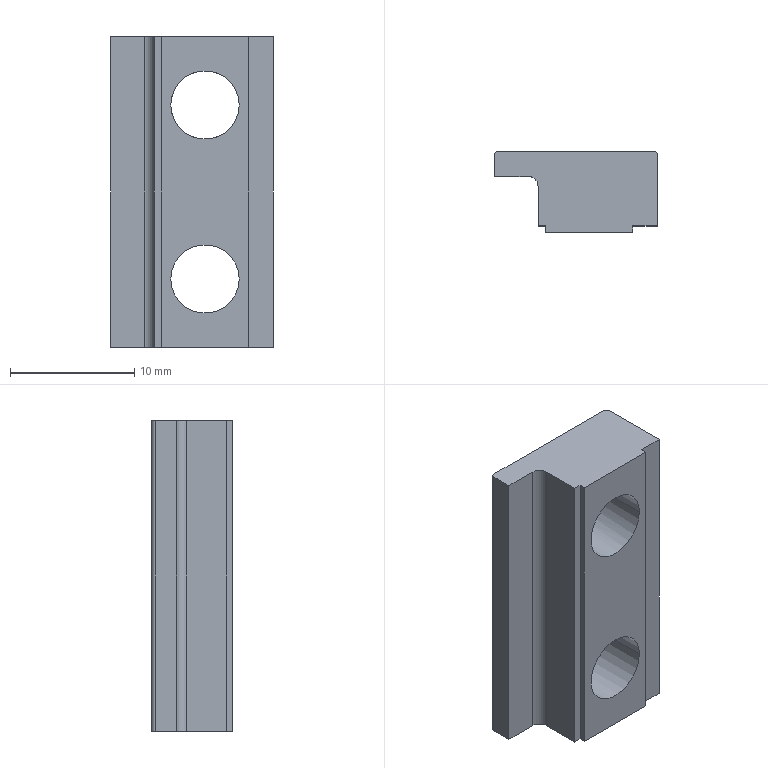Part | SolidWorks | features BaseBody 1 | 1 solid | 23 faces | box 13.1 x 6.5 x 25 mm | volume 1279 mm3 | plane 12 | cylinder 7 | cone 4 | commonest cylinder face diameters 5.5 x4 0.6 x2 1.6 x1
STEP:
#1=CARTESIAN_POINT('',(1.05,0.4528,4.25));
#2=VERTEX_POINT('',#1);
#3=CARTESIAN_POINT('',(-1.7,0.4528,7.));
#4=VERTEX_POINT('',#3);
#5=CARTESIAN_POINT('',(1.05,0.4528,7.));
#6=DIRECTION('',(0.,1.,0.));
#7=DIRECTION('',(0.,0.,1.));
#8=AXIS2_PLACEMENT_3D('',#5,#6,#7);
#9=CIRCLE('',#8,2.75);
#10=EDGE_CURVE('',#2,#4,#9,.T.);
#11=ORIENTED_EDGE('',*,*,#10,.F.);
#12=CARTESIAN_POINT('',(1.05,2.753,1.95));
#13=VERTEX_POINT('',#12);
#14=CARTESIAN_POINT('',(1.05,2.753,1.95));
#15=DIRECTION('',(0.,0.7071,-0.7071));
#16=VECTOR('',#15,1000.);
#17=LINE('',#14,#16);
#18=EDGE_CURVE('',#2,#13,#17,.T.);
#19=ORIENTED_EDGE('',*,*,#18,.T.);
#20=CARTESIAN_POINT('',(1.05,2.753,12.05));
#21=VERTEX_POINT('',#20);
#22=CARTESIAN_POINT('',(1.05,2.753,7.));
#23=DIRECTION('',(0.,-1.,0.));
#24=DIRECTION('',(0.,0.,1.));
#25=AXIS2_PLACEMENT_3D('',#22,#23,#24);
#26=CIRCLE('',#25,5.05);
#27=EDGE_CURVE('',#21,#13,#26,.T.);
#28=ORIENTED_EDGE('',*,*,#27,.F.);
#29=CARTESIAN_POINT('',(1.05,0.4528,9.75));
#30=VERTEX_POINT('',#29);
#31=CARTESIAN_POINT('',(1.05,2.753,12.05));
#32=DIRECTION('',(0.,0.7071,0.7071));
#33=VECTOR('',#32,1000.);
#34=LINE('',#31,#33);
#35=EDGE_CURVE('',#30,#21,#34,.T.);
#36=ORIENTED_EDGE('',*,*,#35,.F.);
#37=CARTESIAN_POINT('',(1.05,0.4528,7.));
#38=DIRECTION('',(0.,1.,0.));
#39=DIRECTION('',(0.,0.,1.));
#40=AXIS2_PLACEMENT_3D('',#37,#38,#39);
#41=CIRCLE('',#40,2.75);
#42=EDGE_CURVE('',#4,#30,#41,.T.);
#43=ORIENTED_EDGE('',*,*,#42,.F.);
#44=EDGE_LOOP('',(#11,#19,#28,#36,#43));
#45=FACE_OUTER_BOUND('',#44,.T.);
#46=CARTESIAN_POINT('',(1.05,2.753,7.));
#47=DIRECTION('',(0.,1.,0.));
#48=DIRECTION('',(0.,0.,1.));
#49=AXIS2_PLACEMENT_3D('',#46,#47,#48);
#50=CONICAL_SURFACE('',#49,5.05,0.7854);
#51=ADVANCED_FACE('',(#45),#50,.F.);
#52=CARTESIAN_POINT('',(3.8,0.4528,-7.));
#53=VERTEX_POINT('',#52);
#54=CARTESIAN_POINT('',(-1.7,0.4528,-7.));
#55=VERTEX_POINT('',#54);
#56=CARTESIAN_POINT('',(1.05,0.4528,-7.));
#57=DIRECTION('',(0.,1.,0.));
#58=DIRECTION('',(-1.,0.,0.));
#59=AXIS2_PLACEMENT_3D('',#56,#57,#58);
#60=CIRCLE('',#59,2.75);
#61=EDGE_CURVE('',#53,#55,#60,.T.);
#62=ORIENTED_EDGE('',*,*,#61,.F.);
#63=CARTESIAN_POINT('',(6.1,2.753,-7.));
#64=VERTEX_POINT('',#63);
#65=CARTESIAN_POINT('',(6.1,2.753,-7.));
#66=DIRECTION('',(0.7071,0.7071,0.));
#67=VECTOR('',#66,1000.);
#68=LINE('',#65,#67);
#69=EDGE_CURVE('',#53,#64,#68,.T.);
#70=ORIENTED_EDGE('',*,*,#69,.T.);
#71=CARTESIAN_POINT('',(-4.,2.753,-7.));
#72=VERTEX_POINT('',#71);
#73=CARTESIAN_POINT('',(1.05,2.753,-7.));
#74=DIRECTION('',(0.,-1.,0.));
#75=DIRECTION('',(-1.,0.,0.));
#76=AXIS2_PLACEMENT_3D('',#73,#74,#75);
#77=CIRCLE('',#76,5.05);
#78=EDGE_CURVE('',#72,#64,#77,.T.);
#79=ORIENTED_EDGE('',*,*,#78,.F.);
#80=CARTESIAN_POINT('',(-4.,2.753,-7.));
#81=DIRECTION('',(-0.7071,0.7071,0.));
#82=VECTOR('',#81,1000.);
#83=LINE('',#80,#82);
#84=EDGE_CURVE('',#55,#72,#83,.T.);
#85=ORIENTED_EDGE('',*,*,#84,.F.);
#86=EDGE_LOOP('',(#62,#70,#79,#85));
#87=FACE_OUTER_BOUND('',#86,.T.);
#88=CARTESIAN_POINT('',(1.05,2.753,-7.));
#89=DIRECTION('',(0.,1.,0.));
#90=DIRECTION('',(-1.,0.,0.));
#91=AXIS2_PLACEMENT_3D('',#88,#89,#90);
#92=CONICAL_SURFACE('',#91,5.05,0.7854);
#93=ADVANCED_FACE('',(#87),#92,.F.);
#94=CARTESIAN_POINT('',(3.8,0.4528,7.));
#95=VERTEX_POINT('',#94);
#96=CARTESIAN_POINT('',(1.05,0.4528,7.));
#97=DIRECTION('',(0.,1.,0.));
#98=DIRECTION('',(0.,0.,1.));
#99=AXIS2_PLACEMENT_3D('',#96,#97,#98);
#100=CIRCLE('',#99,2.75);
#101=EDGE_CURVE('',#95,#2,#100,.T.);
#102=ORIENTED_EDGE('',*,*,#101,.T.);
#103=ORIENTED_EDGE('',*,*,#10,.T.);
#104=CARTESIAN_POINT('',(-1.7,-3.747,7.));
#105=VERTEX_POINT('',#104);
#106=CARTESIAN_POINT('',(-1.7,-3.747,7.));
#107=DIRECTION('',(0.,-1.,0.));
#108=VECTOR('',#107,1000.);
#109=LINE('',#106,#108);
#110=EDGE_CURVE('',#4,#105,#109,.T.);
#111=ORIENTED_EDGE('',*,*,#110,.T.);
#112=CARTESIAN_POINT('',(3.8,-3.747,7.));
#113=VERTEX_POINT('',#112);
#114=CARTESIAN_POINT('',(1.05,-3.747,7.));
#115=DIRECTION('',(0.,1.,0.));
#116=DIRECTION('',(1.,0.,0.));
#117=AXIS2_PLACEMENT_3D('',#114,#115,#116);
#118=CIRCLE('',#117,2.75);
#119=EDGE_CURVE('',#113,#105,#118,.T.);
#120=ORIENTED_EDGE('',*,*,#119,.F.);
#121=CARTESIAN_POINT('',(3.8,-3.747,7.));
#122=DIRECTION('',(0.,-1.,0.));
#123=VECTOR('',#122,1000.);
#124=LINE('',#121,#123);
#125=EDGE_CURVE('',#95,#113,#124,.T.);
#126=ORIENTED_EDGE('',*,*,#125,.F.);
#127=EDGE_LOOP('',(#102,#103,#111,#120,#126));
#128=FACE_OUTER_BOUND('',#127,.T.);
#129=CARTESIAN_POINT('',(1.05,-3.747,7.));
#130=DIRECTION('',(0.,-1.,0.));
#131=DIRECTION('',(1.,0.,0.));
#132=AXIS2_PLACEMENT_3D('',#129,#130,#131);
#133=CYLINDRICAL_SURFACE('',#132,2.75);
#134=ADVANCED_FACE('',(#128),#133,.F.);
#135=ORIENTED_EDGE('',*,*,#61,.T.);
#136=CARTESIAN_POINT('',(-1.7,-3.747,-7.));
#137=VERTEX_POINT('',#136);
#138=CARTESIAN_POINT('',(-1.7,-3.747,-7.));
#139=DIRECTION('',(0.,-1.,0.));
#140=VECTOR('',#139,1000.);
#141=LINE('',#138,#140);
#142=EDGE_CURVE('',#55,#137,#141,.T.);
#143=ORIENTED_EDGE('',*,*,#142,.T.);
#144=CARTESIAN_POINT('',(3.8,-3.747,-7.));
#145=VERTEX_POINT('',#144);
#146=CARTESIAN_POINT('',(1.05,-3.747,-7.));
#147=DIRECTION('',(0.,1.,0.));
#148=DIRECTION('',(1.,0.,0.));
#149=AXIS2_PLACEMENT_3D('',#146,#147,#148);
#150=CIRCLE('',#149,2.75);
#151=EDGE_CURVE('',#145,#137,#150,.T.);
#152=ORIENTED_EDGE('',*,*,#151,.F.);
#153=CARTESIAN_POINT('',(3.8,-3.747,-7.));
#154=DIRECTION('',(0.,-1.,0.));
#155=VECTOR('',#154,1000.);
#156=LINE('',#153,#155);
#157=EDGE_CURVE('',#53,#145,#156,.T.);
#158=ORIENTED_EDGE('',*,*,#157,.F.);
#159=EDGE_LOOP('',(#135,#143,#152,#158));
#160=FACE_OUTER_BOUND('',#159,.T.);
#161=CARTESIAN_POINT('',(1.05,-3.747,-7.));
#162=DIRECTION('',(0.,-1.,0.));
#163=DIRECTION('',(1.,0.,0.));
#164=AXIS2_PLACEMENT_3D('',#161,#162,#163);
#165=CYLINDRICAL_SURFACE('',#164,2.75);
#166=ADVANCED_FACE('',(#160),#165,.F.);
#167=ORIENTED_EDGE('',*,*,#27,.T.);
#168=CARTESIAN_POINT('',(1.05,2.753,7.));
#169=DIRECTION('',(0.,-1.,0.));
#170=DIRECTION('',(0.,0.,1.));
#171=AXIS2_PLACEMENT_3D('',#168,#169,#170);
#172=CIRCLE('',#171,5.05);
#173=EDGE_CURVE('',#13,#21,#172,.T.);
#174=ORIENTED_EDGE('',*,*,#173,.T.);
#175=EDGE_LOOP('',(#167,#174));
#176=FACE_BOUND('',#175,.T.);
#177=ORIENTED_EDGE('',*,*,#78,.T.);
#178=CARTESIAN_POINT('',(1.05,2.753,-7.));
#179=DIRECTION('',(0.,-1.,0.));
#180=DIRECTION('',(-1.,0.,0.));
#181=AXIS2_PLACEMENT_3D('',#178,#179,#180);
#182=CIRCLE('',#181,5.05);
#183=EDGE_CURVE('',#64,#72,#182,.T.);
#184=ORIENTED_EDGE('',*,*,#183,.T.);
#185=EDGE_LOOP('',(#177,#184));
#186=FACE_BOUND('',#185,.T.);
#187=CARTESIAN_POINT('',(6.25,2.753,12.5));
#188=VERTEX_POINT('',#187);
#189=CARTESIAN_POINT('',(6.25,2.753,-12.5));
#190=VERTEX_POINT('',#189);
#191=CARTESIAN_POINT('',(6.25,2.753,-12.5));
#192=DIRECTION('',(0.,0.,-1.));
#193=VECTOR('',#192,1000.);
#194=LINE('',#191,#193);
#195=EDGE_CURVE('',#188,#190,#194,.T.);
#196=ORIENTED_EDGE('',*,*,#195,.T.);
#197=CARTESIAN_POINT('',(-6.25,2.753,-12.5));
#198=VERTEX_POINT('',#197);
#199=CARTESIAN_POINT('',(6.25,2.753,-12.5));
#200=DIRECTION('',(-1.,0.,0.));
#201=VECTOR('',#200,1000.);
#202=LINE('',#199,#201);
#203=EDGE_CURVE('',#190,#198,#202,.T.);
#204=ORIENTED_EDGE('',*,*,#203,.T.);
#205=CARTESIAN_POINT('',(-6.25,2.753,12.5));
#206=VERTEX_POINT('',#205);
#207=CARTESIAN_POINT('',(-6.25,2.753,-12.5));
#208=DIRECTION('',(0.,0.,1.));
#209=VECTOR('',#208,1000.);
#210=LINE('',#207,#209);
#211=EDGE_CURVE('',#198,#206,#210,.T.);
#212=ORIENTED_EDGE('',*,*,#211,.T.);
#213=CARTESIAN_POINT('',(6.25,2.753,12.5));
#214=DIRECTION('',(1.,0.,0.));
#215=VECTOR('',#214,1000.);
#216=LINE('',#213,#215);
#217=EDGE_CURVE('',#206,#188,#216,.T.);
#218=ORIENTED_EDGE('',*,*,#217,.T.);
#219=EDGE_LOOP('',(#196,#204,#212,#218));
#220=FACE_OUTER_BOUND('',#219,.T.);
#221=CARTESIAN_POINT('',(6.25,2.753,-12.5));
#222=DIRECTION('',(0.,1.,0.));
#223=DIRECTION('',(-1.,0.,0.));
#224=AXIS2_PLACEMENT_3D('',#221,#222,#223);
#225=PLANE('',#224);
#226=ADVANCED_FACE('',(#176,#186,#220),#225,.T.);
#227=ORIENTED_EDGE('',*,*,#18,.F.);
#228=ORIENTED_EDGE('',*,*,#101,.F.);
#229=CARTESIAN_POINT('',(1.05,0.4528,7.));
#230=DIRECTION('',(0.,1.,0.));
#231=DIRECTION('',(0.,0.,1.));
#232=AXIS2_PLACEMENT_3D('',#229,#230,#231);
#233=CIRCLE('',#232,2.75);
#234=EDGE_CURVE('',#30,#95,#233,.T.);
#235=ORIENTED_EDGE('',*,*,#234,.F.);
#236=ORIENTED_EDGE('',*,*,#35,.T.);
#237=ORIENTED_EDGE('',*,*,#173,.F.);
#238=EDGE_LOOP('',(#227,#228,#235,#236,#237));
#239=FACE_OUTER_BOUND('',#238,.T.);
#240=CARTESIAN_POINT('',(1.05,2.753,7.));
#241=DIRECTION('',(0.,1.,0.));
#242=DIRECTION('',(0.,0.,1.));
#243=AXIS2_PLACEMENT_3D('',#240,#241,#242);
#244=CONICAL_SURFACE('',#243,5.05,0.7854);
#245=ADVANCED_FACE('',(#239),#244,.F.);
#246=ORIENTED_EDGE('',*,*,#69,.F.);
#247=CARTESIAN_POINT('',(1.05,0.4528,-7.));
#248=DIRECTION('',(0.,1.,0.));
#249=DIRECTION('',(-1.,0.,0.));
#250=AXIS2_PLACEMENT_3D('',#247,#248,#249);
#251=CIRCLE('',#250,2.75);
#252=EDGE_CURVE('',#55,#53,#251,.T.);
#253=ORIENTED_EDGE('',*,*,#252,.F.);
#254=ORIENTED_EDGE('',*,*,#84,.T.);
#255=ORIENTED_EDGE('',*,*,#183,.F.);
#256=EDGE_LOOP('',(#246,#253,#254,#255));
#257=FACE_OUTER_BOUND('',#256,.T.);
#258=CARTESIAN_POINT('',(1.05,2.753,-7.));
#259=DIRECTION('',(0.,1.,0.));
#260=DIRECTION('',(-1.,0.,0.));
#261=AXIS2_PLACEMENT_3D('',#258,#259,#260);
#262=CONICAL_SURFACE('',#261,5.05,0.7854);
#263=ADVANCED_FACE('',(#257),#262,.F.);
#264=CARTESIAN_POINT('',(-3.05,-3.247,-12.5));
#265=VERTEX_POINT('',#264);
#266=CARTESIAN_POINT('',(-2.45,-3.247,-12.5));
#267=VERTEX_POINT('',#266);
#268=CARTESIAN_POINT('',(-3.05,-3.247,-12.5));
#269=DIRECTION('',(1.,0.,0.));
#270=VECTOR('',#269,1000.);
#271=LINE('',#268,#270);
#272=EDGE_CURVE('',#265,#267,#271,.T.);
#273=ORIENTED_EDGE('',*,*,#272,.F.);
#274=CARTESIAN_POINT('',(-3.05,-0.04716,-12.5));
#275=VERTEX_POINT('',#274);
#276=CARTESIAN_POINT('',(-3.05,0.,-12.5));
#277=DIRECTION('',(0.,-1.,0.));
#278=VECTOR('',#277,1000.);
#279=LINE('',#276,#278);
#280=EDGE_CURVE('',#275,#265,#279,.T.);
#281=ORIENTED_EDGE('',*,*,#280,.F.);
#282=CARTESIAN_POINT('',(-3.85,0.7528,-12.5));
#283=VERTEX_POINT('',#282);
#284=CARTESIAN_POINT('',(-3.85,-0.04716,-12.5));
#285=DIRECTION('',(0.,0.,1.));
#286=DIRECTION('',(0.,-1.,0.));
#287=AXIS2_PLACEMENT_3D('',#284,#285,#286);
#288=CIRCLE('',#287,0.8);
#289=EDGE_CURVE('',#275,#283,#288,.T.);
#290=ORIENTED_EDGE('',*,*,#289,.T.);
#291=CARTESIAN_POINT('',(-6.55,0.7528,-12.5));
#292=VERTEX_POINT('',#291);
#293=CARTESIAN_POINT('',(0.,0.7528,-12.5));
#294=DIRECTION('',(1.,0.,0.));
#295=VECTOR('',#294,1000.);
#296=LINE('',#293,#295);
#297=EDGE_CURVE('',#292,#283,#296,.T.);
#298=ORIENTED_EDGE('',*,*,#297,.F.);
#299=CARTESIAN_POINT('',(-6.55,2.453,-12.5));
#300=VERTEX_POINT('',#299);
#301=CARTESIAN_POINT('',(-6.55,2.453,-12.5));
#302=DIRECTION('',(0.,-1.,0.));
#303=VECTOR('',#302,1000.);
#304=LINE('',#301,#303);
#305=EDGE_CURVE('',#300,#292,#304,.T.);
#306=ORIENTED_EDGE('',*,*,#305,.F.);
#307=CARTESIAN_POINT('',(-6.25,2.453,-12.5));
#308=DIRECTION('',(0.,0.,1.));
#309=DIRECTION('',(0.,-1.,0.));
#310=AXIS2_PLACEMENT_3D('',#307,#308,#309);
#311=CIRCLE('',#310,0.3);
#312=EDGE_CURVE('',#198,#300,#311,.T.);
#313=ORIENTED_EDGE('',*,*,#312,.F.);
#314=ORIENTED_EDGE('',*,*,#203,.F.);
#315=CARTESIAN_POINT('',(6.55,2.453,-12.5));
#316=VERTEX_POINT('',#315);
#317=CARTESIAN_POINT('',(6.25,2.453,-12.5));
#318=DIRECTION('',(0.,0.,1.));
#319=DIRECTION('',(0.,-1.,0.));
#320=AXIS2_PLACEMENT_3D('',#317,#318,#319);
#321=CIRCLE('',#320,0.3);
#322=EDGE_CURVE('',#316,#190,#321,.T.);
#323=ORIENTED_EDGE('',*,*,#322,.F.);
#324=CARTESIAN_POINT('',(6.55,-3.247,-12.5));
#325=VERTEX_POINT('',#324);
#326=CARTESIAN_POINT('',(6.55,0.,-12.5));
#327=DIRECTION('',(0.,1.,0.));
#328=VECTOR('',#327,1000.);
#329=LINE('',#326,#328);
#330=EDGE_CURVE('',#325,#316,#329,.T.);
#331=ORIENTED_EDGE('',*,*,#330,.F.);
#332=CARTESIAN_POINT('',(4.55,-3.247,-12.5));
#333=VERTEX_POINT('',#332);
#334=CARTESIAN_POINT('',(0.,-3.247,-12.5));
#335=DIRECTION('',(1.,0.,0.));
#336=VECTOR('',#335,1000.);
#337=LINE('',#334,#336);
#338=EDGE_CURVE('',#333,#325,#337,.T.);
#339=ORIENTED_EDGE('',*,*,#338,.F.);
#340=CARTESIAN_POINT('',(4.55,-3.747,-12.5));
#341=VERTEX_POINT('',#340);
#342=CARTESIAN_POINT('',(4.55,-3.747,-12.5));
#343=DIRECTION('',(0.,1.,0.));
#344=VECTOR('',#343,1000.);
#345=LINE('',#342,#344);
#346=EDGE_CURVE('',#341,#333,#345,.T.);
#347=ORIENTED_EDGE('',*,*,#346,.F.);
#348=CARTESIAN_POINT('',(-2.45,-3.747,-12.5));
#349=VERTEX_POINT('',#348);
#350=CARTESIAN_POINT('',(0.,-3.747,-12.5));
#351=DIRECTION('',(1.,0.,0.));
#352=VECTOR('',#351,1000.);
#353=LINE('',#350,#352);
#354=EDGE_CURVE('',#349,#341,#353,.T.);
#355=ORIENTED_EDGE('',*,*,#354,.F.);
#356=CARTESIAN_POINT('',(-2.45,-3.247,-12.5));
#357=DIRECTION('',(0.,-1.,0.));
#358=VECTOR('',#357,1000.);
#359=LINE('',#356,#358);
#360=EDGE_CURVE('',#267,#349,#359,.T.);
#361=ORIENTED_EDGE('',*,*,#360,.F.);
#362=EDGE_LOOP('',(#273,#281,#290,#298,#306,#313,#314,#323,#331,#339,#347,#355,#361));
#363=FACE_OUTER_BOUND('',#362,.T.);
#364=CARTESIAN_POINT('',(0.,0.,-12.5));
#365=DIRECTION('',(0.,0.,1.));
#366=DIRECTION('',(0.,-1.,0.));
#367=AXIS2_PLACEMENT_3D('',#364,#365,#366);
#368=PLANE('',#367);
#369=ADVANCED_FACE('',(#363),#368,.F.);
#370=CARTESIAN_POINT('',(6.55,2.453,12.5));
#371=VERTEX_POINT('',#370);
#372=CARTESIAN_POINT('',(6.55,2.453,-12.5));
#373=DIRECTION('',(0.,0.,-1.));
#374=VECTOR('',#373,1000.);
#375=LINE('',#372,#374);
#376=EDGE_CURVE('',#371,#316,#375,.T.);
#377=ORIENTED_EDGE('',*,*,#376,.T.);
#378=ORIENTED_EDGE('',*,*,#322,.T.);
#379=ORIENTED_EDGE('',*,*,#195,.F.);
#380=CARTESIAN_POINT('',(6.25,2.453,12.5));
#381=DIRECTION('',(0.,0.,-1.));
#382=DIRECTION('',(0.,-1.,0.));
#383=AXIS2_PLACEMENT_3D('',#380,#381,#382);
#384=CIRCLE('',#383,0.3);
#385=EDGE_CURVE('',#188,#371,#384,.T.);
#386=ORIENTED_EDGE('',*,*,#385,.T.);
#387=EDGE_LOOP('',(#377,#378,#379,#386));
#388=FACE_OUTER_BOUND('',#387,.T.);
#389=CARTESIAN_POINT('',(6.25,2.453,-12.5));
#390=DIRECTION('',(0.,0.,1.));
#391=DIRECTION('',(0.,-1.,0.));
#392=AXIS2_PLACEMENT_3D('',#389,#390,#391);
#393=CYLINDRICAL_SURFACE('',#392,0.3);
#394=ADVANCED_FACE('',(#388),#393,.T.);
#395=CARTESIAN_POINT('',(-3.05,-0.04716,12.5));
#396=VERTEX_POINT('',#395);
#397=CARTESIAN_POINT('',(-3.05,-3.247,12.5));
#398=VERTEX_POINT('',#397);
#399=CARTESIAN_POINT('',(-3.05,0.,12.5));
#400=DIRECTION('',(0.,-1.,0.));
#401=VECTOR('',#400,1000.);
#402=LINE('',#399,#401);
#403=EDGE_CURVE('',#396,#398,#402,.T.);
#404=ORIENTED_EDGE('',*,*,#403,.T.);
#405=CARTESIAN_POINT('',(-2.45,-3.247,12.5));
#406=VERTEX_POINT('',#405);
#407=CARTESIAN_POINT('',(-3.05,-3.247,12.5));
#408=DIRECTION('',(-1.,0.,0.));
#409=VECTOR('',#408,1000.);
#410=LINE('',#407,#409);
#411=EDGE_CURVE('',#406,#398,#410,.T.);
#412=ORIENTED_EDGE('',*,*,#411,.F.);
#413=CARTESIAN_POINT('',(-2.45,-3.747,12.5));
#414=VERTEX_POINT('',#413);
#415=CARTESIAN_POINT('',(-2.45,-3.247,12.5));
#416=DIRECTION('',(0.,1.,0.));
#417=VECTOR('',#416,1000.);
#418=LINE('',#415,#417);
#419=EDGE_CURVE('',#414,#406,#418,.T.);
#420=ORIENTED_EDGE('',*,*,#419,.F.);
#421=CARTESIAN_POINT('',(4.55,-3.747,12.5));
#422=VERTEX_POINT('',#421);
#423=CARTESIAN_POINT('',(0.,-3.747,12.5));
#424=DIRECTION('',(1.,0.,0.));
#425=VECTOR('',#424,1000.);
#426=LINE('',#423,#425);
#427=EDGE_CURVE('',#414,#422,#426,.T.);
#428=ORIENTED_EDGE('',*,*,#427,.T.);
#429=CARTESIAN_POINT('',(4.55,-3.247,12.5));
#430=VERTEX_POINT('',#429);
#431=CARTESIAN_POINT('',(4.55,-3.747,12.5));
#432=DIRECTION('',(0.,-1.,0.));
#433=VECTOR('',#432,1000.);
#434=LINE('',#431,#433);
#435=EDGE_CURVE('',#430,#422,#434,.T.);
#436=ORIENTED_EDGE('',*,*,#435,.F.);
#437=CARTESIAN_POINT('',(6.55,-3.247,12.5));
#438=VERTEX_POINT('',#437);
#439=CARTESIAN_POINT('',(0.,-3.247,12.5));
#440=DIRECTION('',(1.,0.,0.));
#441=VECTOR('',#440,1000.);
#442=LINE('',#439,#441);
#443=EDGE_CURVE('',#430,#438,#442,.T.);
#444=ORIENTED_EDGE('',*,*,#443,.T.);
#445=CARTESIAN_POINT('',(6.55,0.,12.5));
#446=DIRECTION('',(0.,1.,0.));
#447=VECTOR('',#446,1000.);
#448=LINE('',#445,#447);
#449=EDGE_CURVE('',#438,#371,#448,.T.);
#450=ORIENTED_EDGE('',*,*,#449,.T.);
#451=ORIENTED_EDGE('',*,*,#385,.F.);
#452=ORIENTED_EDGE('',*,*,#217,.F.);
#453=CARTESIAN_POINT('',(-6.55,2.453,12.5));
#454=VERTEX_POINT('',#453);
#455=CARTESIAN_POINT('',(-6.25,2.453,12.5));
#456=DIRECTION('',(0.,0.,1.));
#457=DIRECTION('',(0.,-1.,0.));
#458=AXIS2_PLACEMENT_3D('',#455,#456,#457);
#459=CIRCLE('',#458,0.3);
#460=EDGE_CURVE('',#206,#454,#459,.T.);
#461=ORIENTED_EDGE('',*,*,#460,.T.);
#462=CARTESIAN_POINT('',(-6.55,0.7528,12.5));
#463=VERTEX_POINT('',#462);
#464=CARTESIAN_POINT('',(-6.55,2.453,12.5));
#465=DIRECTION('',(0.,1.,0.));
#466=VECTOR('',#465,1000.);
#467=LINE('',#464,#466);
#468=EDGE_CURVE('',#463,#454,#467,.T.);
#469=ORIENTED_EDGE('',*,*,#468,.F.);
#470=CARTESIAN_POINT('',(-3.85,0.7528,12.5));
#471=VERTEX_POINT('',#470);
#472=CARTESIAN_POINT('',(0.,0.7528,12.5));
#473=DIRECTION('',(1.,0.,0.));
#474=VECTOR('',#473,1000.);
#475=LINE('',#472,#474);
#476=EDGE_CURVE('',#463,#471,#475,.T.);
#477=ORIENTED_EDGE('',*,*,#476,.T.);
#478=CARTESIAN_POINT('',(-3.85,-0.04716,12.5));
#479=DIRECTION('',(0.,0.,-1.));
#480=DIRECTION('',(0.,-1.,0.));
#481=AXIS2_PLACEMENT_3D('',#478,#479,#480);
#482=CIRCLE('',#481,0.8);
#483=EDGE_CURVE('',#471,#396,#482,.T.);
#484=ORIENTED_EDGE('',*,*,#483,.T.);
#485=EDGE_LOOP('',(#404,#412,#420,#428,#436,#444,#450,#451,#452,#461,#469,#477,#484));
#486=FACE_OUTER_BOUND('',#485,.T.);
#487=CARTESIAN_POINT('',(0.,0.,12.5));
#488=DIRECTION('',(0.,0.,1.));
#489=DIRECTION('',(0.,-1.,0.));
#490=AXIS2_PLACEMENT_3D('',#487,#488,#489);
#491=PLANE('',#490);
#492=ADVANCED_FACE('',(#486),#491,.T.);
#493=ORIENTED_EDGE('',*,*,#211,.F.);
#494=ORIENTED_EDGE('',*,*,#312,.T.);
#495=CARTESIAN_POINT('',(-6.55,2.453,-12.5));
#496=DIRECTION('',(0.,0.,1.));
#497=VECTOR('',#496,1000.);
#498=LINE('',#495,#497);
#499=EDGE_CURVE('',#300,#454,#498,.T.);
#500=ORIENTED_EDGE('',*,*,#499,.T.);
#501=ORIENTED_EDGE('',*,*,#460,.F.);
#502=EDGE_LOOP('',(#493,#494,#500,#501));
#503=FACE_OUTER_BOUND('',#502,.T.);
#504=CARTESIAN_POINT('',(-6.25,2.453,-12.5));
#505=DIRECTION('',(0.,0.,1.));
#506=DIRECTION('',(0.,-1.,0.));
#507=AXIS2_PLACEMENT_3D('',#504,#505,#506);
#508=CYLINDRICAL_SURFACE('',#507,0.3);
#509=ADVANCED_FACE('',(#503),#508,.T.);
#510=ORIENTED_EDGE('',*,*,#110,.F.);
#511=ORIENTED_EDGE('',*,*,#42,.T.);
#512=ORIENTED_EDGE('',*,*,#234,.T.);
#513=ORIENTED_EDGE('',*,*,#125,.T.);
#514=CARTESIAN_POINT('',(1.05,-3.747,7.));
#515=DIRECTION('',(0.,1.,0.));
#516=DIRECTION('',(1.,0.,0.));
#517=AXIS2_PLACEMENT_3D('',#514,#515,#516);
#518=CIRCLE('',#517,2.75);
#519=EDGE_CURVE('',#105,#113,#518,.T.);
#520=ORIENTED_EDGE('',*,*,#519,.F.);
#521=EDGE_LOOP('',(#510,#511,#512,#513,#520));
#522=FACE_OUTER_BOUND('',#521,.T.);
#523=CARTESIAN_POINT('',(1.05,-3.747,7.));
#524=DIRECTION('',(0.,-1.,0.));
#525=DIRECTION('',(1.,0.,0.));
#526=AXIS2_PLACEMENT_3D('',#523,#524,#525);
#527=CYLINDRICAL_SURFACE('',#526,2.75);
#528=ADVANCED_FACE('',(#522),#527,.F.);
#529=ORIENTED_EDGE('',*,*,#142,.F.);
#530=ORIENTED_EDGE('',*,*,#252,.T.);
#531=ORIENTED_EDGE('',*,*,#157,.T.);
#532=CARTESIAN_POINT('',(1.05,-3.747,-7.));
#533=DIRECTION('',(0.,1.,0.));
#534=DIRECTION('',(1.,0.,0.));
#535=AXIS2_PLACEMENT_3D('',#532,#533,#534);
#536=CIRCLE('',#535,2.75);
#537=EDGE_CURVE('',#137,#145,#536,.T.);
#538=ORIENTED_EDGE('',*,*,#537,.F.);
#539=EDGE_LOOP('',(#529,#530,#531,#538));
#540=FACE_OUTER_BOUND('',#539,.T.);
#541=CARTESIAN_POINT('',(1.05,-3.747,-7.));
#542=DIRECTION('',(0.,-1.,0.));
#543=DIRECTION('',(1.,0.,0.));
#544=AXIS2_PLACEMENT_3D('',#541,#542,#543);
#545=CYLINDRICAL_SURFACE('',#544,2.75);
#546=ADVANCED_FACE('',(#540),#545,.F.);
#547=CARTESIAN_POINT('',(-3.05,-0.04716,-12.5));
#548=DIRECTION('',(0.,0.,-1.));
#549=VECTOR('',#548,1000.);
#550=LINE('',#547,#549);
#551=EDGE_CURVE('',#396,#275,#550,.T.);
#552=ORIENTED_EDGE('',*,*,#551,.T.);
#553=ORIENTED_EDGE('',*,*,#280,.T.);
#554=CARTESIAN_POINT('',(-3.05,-3.247,-12.5));
#555=DIRECTION('',(0.,0.,1.));
#556=VECTOR('',#555,1000.);
#557=LINE('',#554,#556);
#558=EDGE_CURVE('',#265,#398,#557,.T.);
#559=ORIENTED_EDGE('',*,*,#558,.T.);
#560=ORIENTED_EDGE('',*,*,#403,.F.);
#561=EDGE_LOOP('',(#552,#553,#559,#560));
#562=FACE_OUTER_BOUND('',#561,.T.);
#563=CARTESIAN_POINT('',(-3.05,-0.04716,-12.5));
#564=DIRECTION('',(-1.,0.,0.));
#565=DIRECTION('',(0.,-1.,0.));
#566=AXIS2_PLACEMENT_3D('',#563,#564,#565);
#567=PLANE('',#566);
#568=ADVANCED_FACE('',(#562),#567,.T.);
#569=CARTESIAN_POINT('',(-6.55,0.7528,-12.5));
#570=DIRECTION('',(0.,0.,-1.));
#571=VECTOR('',#570,1000.);
#572=LINE('',#569,#571);
#573=EDGE_CURVE('',#463,#292,#572,.T.);
#574=ORIENTED_EDGE('',*,*,#573,.T.);
#575=ORIENTED_EDGE('',*,*,#297,.T.);
#576=CARTESIAN_POINT('',(-3.85,0.7528,-12.5));
#577=DIRECTION('',(0.,0.,1.));
#578=VECTOR('',#577,1000.);
#579=LINE('',#576,#578);
#580=EDGE_CURVE('',#283,#471,#579,.T.);
#581=ORIENTED_EDGE('',*,*,#580,.T.);
#582=ORIENTED_EDGE('',*,*,#476,.F.);
#583=EDGE_LOOP('',(#574,#575,#581,#582));
#584=FACE_OUTER_BOUND('',#583,.T.);
#585=CARTESIAN_POINT('',(-6.55,0.7528,-12.5));
#586=DIRECTION('',(0.,-1.,0.));
#587=DIRECTION('',(1.,0.,0.));
#588=AXIS2_PLACEMENT_3D('',#585,#586,#587);
#589=PLANE('',#588);
#590=ADVANCED_FACE('',(#584),#589,.T.);
#591=CARTESIAN_POINT('',(6.55,-3.247,-12.5));
#592=DIRECTION('',(0.,0.,-1.));
#593=VECTOR('',#592,1000.);
#594=LINE('',#591,#593);
#595=EDGE_CURVE('',#438,#325,#594,.T.);
#596=ORIENTED_EDGE('',*,*,#595,.T.);
#597=ORIENTED_EDGE('',*,*,#330,.T.);
#598=ORIENTED_EDGE('',*,*,#376,.F.);
#599=ORIENTED_EDGE('',*,*,#449,.F.);
#600=EDGE_LOOP('',(#596,#597,#598,#599));
#601=FACE_OUTER_BOUND('',#600,.T.);
#602=CARTESIAN_POINT('',(6.55,-3.247,-12.5));
#603=DIRECTION('',(1.,0.,0.));
#604=DIRECTION('',(0.,1.,0.));
#605=AXIS2_PLACEMENT_3D('',#602,#603,#604);
#606=PLANE('',#605);
#607=ADVANCED_FACE('',(#601),#606,.T.);
#608=CARTESIAN_POINT('',(4.55,-3.247,-12.5));
#609=DIRECTION('',(0.,0.,-1.));
#610=VECTOR('',#609,1000.);
#611=LINE('',#608,#610);
#612=EDGE_CURVE('',#430,#333,#611,.T.);
#613=ORIENTED_EDGE('',*,*,#612,.T.);
#614=ORIENTED_EDGE('',*,*,#338,.T.);
#615=ORIENTED_EDGE('',*,*,#595,.F.);
#616=ORIENTED_EDGE('',*,*,#443,.F.);
#617=EDGE_LOOP('',(#613,#614,#615,#616));
#618=FACE_OUTER_BOUND('',#617,.T.);
#619=CARTESIAN_POINT('',(4.55,-3.247,-12.5));
#620=DIRECTION('',(0.,-1.,0.));
#621=DIRECTION('',(1.,0.,0.));
#622=AXIS2_PLACEMENT_3D('',#619,#620,#621);
#623=PLANE('',#622);
#624=ADVANCED_FACE('',(#618),#623,.T.);
#625=ORIENTED_EDGE('',*,*,#151,.T.);
#626=ORIENTED_EDGE('',*,*,#537,.T.);
#627=EDGE_LOOP('',(#625,#626));
#628=FACE_BOUND('',#627,.T.);
#629=ORIENTED_EDGE('',*,*,#119,.T.);
#630=ORIENTED_EDGE('',*,*,#519,.T.);
#631=EDGE_LOOP('',(#629,#630));
#632=FACE_BOUND('',#631,.T.);
#633=CARTESIAN_POINT('',(-2.45,-3.747,-12.5));
#634=DIRECTION('',(0.,0.,-1.));
#635=VECTOR('',#634,1000.);
#636=LINE('',#633,#635);
#637=EDGE_CURVE('',#414,#349,#636,.T.);
#638=ORIENTED_EDGE('',*,*,#637,.T.);
#639=ORIENTED_EDGE('',*,*,#354,.T.);
#640=CARTESIAN_POINT('',(4.55,-3.747,-12.5));
#641=DIRECTION('',(0.,0.,1.));
#642=VECTOR('',#641,1000.);
#643=LINE('',#640,#642);
#644=EDGE_CURVE('',#341,#422,#643,.T.);
#645=ORIENTED_EDGE('',*,*,#644,.T.);
#646=ORIENTED_EDGE('',*,*,#427,.F.);
#647=EDGE_LOOP('',(#638,#639,#645,#646));
#648=FACE_OUTER_BOUND('',#647,.T.);
#649=CARTESIAN_POINT('',(-2.45,-3.747,-12.5));
#650=DIRECTION('',(0.,-1.,0.));
#651=DIRECTION('',(1.,0.,0.));
#652=AXIS2_PLACEMENT_3D('',#649,#650,#651);
#653=PLANE('',#652);
#654=ADVANCED_FACE('',(#628,#632,#648),#653,.T.);
#655=ORIENTED_EDGE('',*,*,#499,.F.);
#656=ORIENTED_EDGE('',*,*,#305,.T.);
#657=ORIENTED_EDGE('',*,*,#573,.F.);
#658=ORIENTED_EDGE('',*,*,#468,.T.);
#659=EDGE_LOOP('',(#655,#656,#657,#658));
#660=FACE_OUTER_BOUND('',#659,.T.);
#661=CARTESIAN_POINT('',(-6.55,2.453,-12.5));
#662=DIRECTION('',(-1.,0.,0.));
#663=DIRECTION('',(0.,-1.,0.));
#664=AXIS2_PLACEMENT_3D('',#661,#662,#663);
#665=PLANE('',#664);
#666=ADVANCED_FACE('',(#660),#665,.T.);
#667=ORIENTED_EDGE('',*,*,#289,.F.);
#668=ORIENTED_EDGE('',*,*,#551,.F.);
#669=ORIENTED_EDGE('',*,*,#483,.F.);
#670=ORIENTED_EDGE('',*,*,#580,.F.);
#671=EDGE_LOOP('',(#667,#668,#669,#670));
#672=FACE_OUTER_BOUND('',#671,.T.);
#673=CARTESIAN_POINT('',(-3.85,-0.04716,-12.5));
#674=DIRECTION('',(0.,0.,1.));
#675=DIRECTION('',(0.,-1.,0.));
#676=AXIS2_PLACEMENT_3D('',#673,#674,#675);
#677=CYLINDRICAL_SURFACE('',#676,0.8);
#678=ADVANCED_FACE('',(#672),#677,.F.);
#679=ORIENTED_EDGE('',*,*,#558,.F.);
#680=ORIENTED_EDGE('',*,*,#272,.T.);
#681=CARTESIAN_POINT('',(-2.45,-3.247,-12.5));
#682=DIRECTION('',(0.,0.,1.));
#683=VECTOR('',#682,1000.);
#684=LINE('',#681,#683);
#685=EDGE_CURVE('',#267,#406,#684,.T.);
#686=ORIENTED_EDGE('',*,*,#685,.T.);
#687=ORIENTED_EDGE('',*,*,#411,.T.);
#688=EDGE_LOOP('',(#679,#680,#686,#687));
#689=FACE_OUTER_BOUND('',#688,.T.);
#690=CARTESIAN_POINT('',(-3.05,-3.247,-12.5));
#691=DIRECTION('',(0.,-1.,0.));
#692=DIRECTION('',(1.,0.,0.));
#693=AXIS2_PLACEMENT_3D('',#690,#691,#692);
#694=PLANE('',#693);
#695=ADVANCED_FACE('',(#689),#694,.T.);
#696=ORIENTED_EDGE('',*,*,#644,.F.);
#697=ORIENTED_EDGE('',*,*,#346,.T.);
#698=ORIENTED_EDGE('',*,*,#612,.F.);
#699=ORIENTED_EDGE('',*,*,#435,.T.);
#700=EDGE_LOOP('',(#696,#697,#698,#699));
#701=FACE_OUTER_BOUND('',#700,.T.);
#702=CARTESIAN_POINT('',(4.55,-3.747,-12.5));
#703=DIRECTION('',(1.,0.,0.));
#704=DIRECTION('',(0.,1.,0.));
#705=AXIS2_PLACEMENT_3D('',#702,#703,#704);
#706=PLANE('',#705);
#707=ADVANCED_FACE('',(#701),#706,.T.);
#708=ORIENTED_EDGE('',*,*,#685,.F.);
#709=ORIENTED_EDGE('',*,*,#360,.T.);
#710=ORIENTED_EDGE('',*,*,#637,.F.);
#711=ORIENTED_EDGE('',*,*,#419,.T.);
#712=EDGE_LOOP('',(#708,#709,#710,#711));
#713=FACE_OUTER_BOUND('',#712,.T.);
#714=CARTESIAN_POINT('',(-2.45,-3.247,-12.5));
#715=DIRECTION('',(-1.,0.,0.));
#716=DIRECTION('',(0.,-1.,0.));
#717=AXIS2_PLACEMENT_3D('',#714,#715,#716);
#718=PLANE('',#717);
#719=ADVANCED_FACE('',(#713),#718,.T.);
#720=CLOSED_SHELL('',(#51,#93,#134,#166,#226,#245,#263,#369,#394,#492,#509,#528,#546,#568,#590,#607,#624,#654,#666,#678,#695,#707,#719));
#721=MANIFOLD_SOLID_BREP('',#720);
#722=CARTESIAN_POINT('',(0.,0.,0.));
#723=DIRECTION('',(0.,0.,1.));
#724=DIRECTION('',(1.,0.,0.));
#725=AXIS2_PLACEMENT_3D('',#722,#723,#724);
#726=(LENGTH_UNIT()NAMED_UNIT(*)SI_UNIT(.MILLI.,.METRE.));
#727=UNCERTAINTY_MEASURE_WITH_UNIT(LENGTH_MEASURE(0.00001),#726,'','');
#728=(NAMED_UNIT(*)PLANE_ANGLE_UNIT()SI_UNIT($,.RADIAN.));
#729=(NAMED_UNIT(*)SI_UNIT($,.STERADIAN.)SOLID_ANGLE_UNIT());
#730=(GEOMETRIC_REPRESENTATION_CONTEXT(3)GLOBAL_UNCERTAINTY_ASSIGNED_CONTEXT((#727))GLOBAL_UNIT_ASSIGNED_CONTEXT((#726,#728,#729))REPRESENTATION_CONTEXT('',''));
#731=ADVANCED_BREP_SHAPE_REPRESENTATION('',(#721,#725),#730);